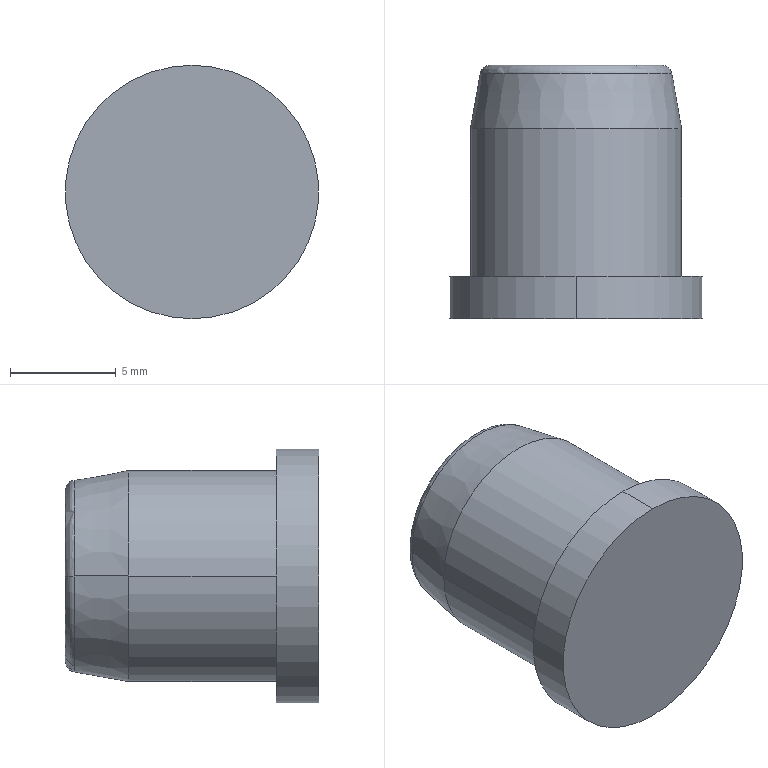Part | STEP file | 1519D3-2.stp.STEP | 1 solid | 12 faces | box 12 x 12 x 12 mm | volume 986.571 mm3 | cylinder 4 | plane 3 | cone 3 | torus 2 | commonest cylinder face diameters 10 x2 12 x2
STEP:
#1=CARTESIAN_POINT('',(0.,0.,6.));
#2=VERTEX_POINT('',#1);
#3=CARTESIAN_POINT('',(0.,0.,-6.));
#4=VERTEX_POINT('',#3);
#5=CARTESIAN_POINT('',(0.,0.,0.));
#6=DIRECTION('',(0.,-1.,0.));
#7=DIRECTION('',(0.,0.,1.));
#8=AXIS2_PLACEMENT_3D('',#5,#6,#7);
#9=CIRCLE('',#8,6.);
#10=EDGE_CURVE('',#2,#4,#9,.T.);
#11=ORIENTED_EDGE('',*,*,#10,.T.);
#12=CARTESIAN_POINT('',(0.,0.,0.));
#13=DIRECTION('',(0.,-1.,0.));
#14=DIRECTION('',(0.,0.,-1.));
#15=AXIS2_PLACEMENT_3D('',#12,#13,#14);
#16=CIRCLE('',#15,6.);
#17=EDGE_CURVE('',#4,#2,#16,.T.);
#18=ORIENTED_EDGE('',*,*,#17,.T.);
#19=EDGE_LOOP('',(#11,#18));
#20=FACE_OUTER_BOUND('',#19,.T.);
#21=CARTESIAN_POINT('',(0.,0.,0.));
#22=DIRECTION('',(0.,1.,0.));
#23=DIRECTION('',(1.,0.,0.));
#24=AXIS2_PLACEMENT_3D('',#21,#22,#23);
#25=PLANE('',#24);
#26=ADVANCED_FACE('',(#20),#25,.F.);
#27=CARTESIAN_POINT('',(0.,2.,-6.));
#28=VERTEX_POINT('',#27);
#29=CARTESIAN_POINT('',(0.,0.,-6.));
#30=DIRECTION('',(0.,1.,0.));
#31=VECTOR('',#30,1000.);
#32=LINE('',#29,#31);
#33=EDGE_CURVE('',#4,#28,#32,.T.);
#34=ORIENTED_EDGE('',*,*,#33,.T.);
#35=CARTESIAN_POINT('',(0.,2.,6.));
#36=VERTEX_POINT('',#35);
#37=CARTESIAN_POINT('',(0.,2.,0.));
#38=DIRECTION('',(0.,-1.,0.));
#39=DIRECTION('',(0.,0.,-1.));
#40=AXIS2_PLACEMENT_3D('',#37,#38,#39);
#41=CIRCLE('',#40,6.);
#42=EDGE_CURVE('',#28,#36,#41,.T.);
#43=ORIENTED_EDGE('',*,*,#42,.T.);
#44=CARTESIAN_POINT('',(0.,0.,6.));
#45=DIRECTION('',(0.,1.,0.));
#46=VECTOR('',#45,1000.);
#47=LINE('',#44,#46);
#48=EDGE_CURVE('',#2,#36,#47,.T.);
#49=ORIENTED_EDGE('',*,*,#48,.F.);
#50=ORIENTED_EDGE('',*,*,#17,.F.);
#51=EDGE_LOOP('',(#34,#43,#49,#50));
#52=FACE_OUTER_BOUND('',#51,.T.);
#53=CARTESIAN_POINT('',(0.,0.,0.));
#54=DIRECTION('',(0.,-1.,0.));
#55=DIRECTION('',(0.,0.,-1.));
#56=AXIS2_PLACEMENT_3D('',#53,#54,#55);
#57=CYLINDRICAL_SURFACE('',#56,6.);
#58=ADVANCED_FACE('',(#52),#57,.T.);
#59=ORIENTED_EDGE('',*,*,#48,.T.);
#60=CARTESIAN_POINT('',(0.,2.,0.));
#61=DIRECTION('',(0.,-1.,0.));
#62=DIRECTION('',(0.,0.,1.));
#63=AXIS2_PLACEMENT_3D('',#60,#61,#62);
#64=CIRCLE('',#63,6.);
#65=EDGE_CURVE('',#36,#28,#64,.T.);
#66=ORIENTED_EDGE('',*,*,#65,.T.);
#67=ORIENTED_EDGE('',*,*,#33,.F.);
#68=ORIENTED_EDGE('',*,*,#10,.F.);
#69=EDGE_LOOP('',(#59,#66,#67,#68));
#70=FACE_OUTER_BOUND('',#69,.T.);
#71=CARTESIAN_POINT('',(0.,0.,0.));
#72=DIRECTION('',(0.,-1.,0.));
#73=DIRECTION('',(0.,0.,-1.));
#74=AXIS2_PLACEMENT_3D('',#71,#72,#73);
#75=CYLINDRICAL_SURFACE('',#74,6.);
#76=ADVANCED_FACE('',(#70),#75,.T.);
#77=CARTESIAN_POINT('',(-5.,2.,0.));
#78=VERTEX_POINT('',#77);
#79=CARTESIAN_POINT('',(5.,2.,0.));
#80=VERTEX_POINT('',#79);
#81=CARTESIAN_POINT('',(0.,2.,0.));
#82=DIRECTION('',(0.,1.,0.));
#83=DIRECTION('',(-1.,0.,0.));
#84=AXIS2_PLACEMENT_3D('',#81,#82,#83);
#85=CIRCLE('',#84,5.);
#86=EDGE_CURVE('',#78,#80,#85,.T.);
#87=ORIENTED_EDGE('',*,*,#86,.F.);
#88=CARTESIAN_POINT('',(0.,2.,0.));
#89=DIRECTION('',(0.,1.,0.));
#90=DIRECTION('',(1.,0.,0.));
#91=AXIS2_PLACEMENT_3D('',#88,#89,#90);
#92=CIRCLE('',#91,5.);
#93=EDGE_CURVE('',#80,#78,#92,.T.);
#94=ORIENTED_EDGE('',*,*,#93,.F.);
#95=EDGE_LOOP('',(#87,#94));
#96=FACE_BOUND('',#95,.T.);
#97=ORIENTED_EDGE('',*,*,#65,.F.);
#98=ORIENTED_EDGE('',*,*,#42,.F.);
#99=EDGE_LOOP('',(#97,#98));
#100=FACE_OUTER_BOUND('',#99,.T.);
#101=CARTESIAN_POINT('',(0.,2.,0.));
#102=DIRECTION('',(0.,-1.,0.));
#103=DIRECTION('',(0.,0.,-1.));
#104=AXIS2_PLACEMENT_3D('',#101,#102,#103);
#105=PLANE('',#104);
#106=ADVANCED_FACE('',(#96,#100),#105,.F.);
#107=CARTESIAN_POINT('',(-5.,9.,0.));
#108=VERTEX_POINT('',#107);
#109=CARTESIAN_POINT('',(-5.,2.,0.));
#110=DIRECTION('',(0.,1.,0.));
#111=VECTOR('',#110,1000.);
#112=LINE('',#109,#111);
#113=EDGE_CURVE('',#78,#108,#112,.T.);
#114=ORIENTED_EDGE('',*,*,#113,.T.);
#115=CARTESIAN_POINT('',(0.,9.,-5.));
#116=VERTEX_POINT('',#115);
#117=CARTESIAN_POINT('',(0.,9.,0.));
#118=DIRECTION('',(0.,1.,0.));
#119=DIRECTION('',(1.,0.,0.));
#120=AXIS2_PLACEMENT_3D('',#117,#118,#119);
#121=CIRCLE('',#120,5.);
#122=EDGE_CURVE('',#116,#108,#121,.T.);
#123=ORIENTED_EDGE('',*,*,#122,.F.);
#124=CARTESIAN_POINT('',(5.,9.,0.));
#125=VERTEX_POINT('',#124);
#126=CARTESIAN_POINT('',(0.,9.,0.));
#127=DIRECTION('',(0.,1.,0.));
#128=DIRECTION('',(1.,0.,0.));
#129=AXIS2_PLACEMENT_3D('',#126,#127,#128);
#130=CIRCLE('',#129,5.);
#131=EDGE_CURVE('',#125,#116,#130,.T.);
#132=ORIENTED_EDGE('',*,*,#131,.F.);
#133=CARTESIAN_POINT('',(5.,2.,0.));
#134=DIRECTION('',(0.,1.,0.));
#135=VECTOR('',#134,1000.);
#136=LINE('',#133,#135);
#137=EDGE_CURVE('',#80,#125,#136,.T.);
#138=ORIENTED_EDGE('',*,*,#137,.F.);
#139=ORIENTED_EDGE('',*,*,#93,.T.);
#140=EDGE_LOOP('',(#114,#123,#132,#138,#139));
#141=FACE_OUTER_BOUND('',#140,.T.);
#142=CARTESIAN_POINT('',(0.,0.,0.));
#143=DIRECTION('',(0.,1.,0.));
#144=DIRECTION('',(1.,0.,0.));
#145=AXIS2_PLACEMENT_3D('',#142,#143,#144);
#146=CYLINDRICAL_SURFACE('',#145,5.);
#147=ADVANCED_FACE('',(#141),#146,.T.);
#148=ORIENTED_EDGE('',*,*,#137,.T.);
#149=CARTESIAN_POINT('',(0.,9.,0.));
#150=DIRECTION('',(0.,1.,0.));
#151=DIRECTION('',(-1.,0.,0.));
#152=AXIS2_PLACEMENT_3D('',#149,#150,#151);
#153=CIRCLE('',#152,5.);
#154=EDGE_CURVE('',#108,#125,#153,.T.);
#155=ORIENTED_EDGE('',*,*,#154,.F.);
#156=ORIENTED_EDGE('',*,*,#113,.F.);
#157=ORIENTED_EDGE('',*,*,#86,.T.);
#158=EDGE_LOOP('',(#148,#155,#156,#157));
#159=FACE_OUTER_BOUND('',#158,.T.);
#160=CARTESIAN_POINT('',(0.,0.,0.));
#161=DIRECTION('',(0.,1.,0.));
#162=DIRECTION('',(1.,0.,0.));
#163=AXIS2_PLACEMENT_3D('',#160,#161,#162);
#164=CYLINDRICAL_SURFACE('',#163,5.);
#165=ADVANCED_FACE('',(#159),#164,.T.);
#166=CARTESIAN_POINT('',(-4.544,11.587,0.000000001));
#167=VERTEX_POINT('',#166);
#168=CARTESIAN_POINT('',(-4.544,11.587,-0.000000004));
#169=DIRECTION('',(-0.1736,-0.9848,0.000000002));
#170=VECTOR('',#169,1000.);
#171=LINE('',#168,#170);
#172=EDGE_CURVE('',#167,#108,#171,.T.);
#173=ORIENTED_EDGE('',*,*,#172,.T.);
#174=ORIENTED_EDGE('',*,*,#154,.T.);
#175=CARTESIAN_POINT('',(4.544,11.587,-0.000000001));
#176=VERTEX_POINT('',#175);
#177=CARTESIAN_POINT('',(4.544,11.587,0.000000004));
#178=DIRECTION('',(0.1736,-0.9848,-0.000000002));
#179=VECTOR('',#178,1000.);
#180=LINE('',#177,#179);
#181=EDGE_CURVE('',#176,#125,#180,.T.);
#182=ORIENTED_EDGE('',*,*,#181,.F.);
#183=CARTESIAN_POINT('',(0.,11.587,0.));
#184=DIRECTION('',(0.,1.,0.));
#185=DIRECTION('',(-1.,0.,0.));
#186=AXIS2_PLACEMENT_3D('',#183,#184,#185);
#187=CIRCLE('',#186,4.544);
#188=EDGE_CURVE('',#167,#176,#187,.T.);
#189=ORIENTED_EDGE('',*,*,#188,.F.);
#190=EDGE_LOOP('',(#173,#174,#182,#189));
#191=FACE_OUTER_BOUND('',#190,.T.);
#192=CARTESIAN_POINT('',(0.,10.293,0.));
#193=DIRECTION('',(0.,-1.,0.));
#194=DIRECTION('',(0.,0.,-1.));
#195=AXIS2_PLACEMENT_3D('',#192,#193,#194);
#196=CONICAL_SURFACE('',#195,4.772,0.1745);
#197=ADVANCED_FACE('',(#191),#196,.T.);
#198=CARTESIAN_POINT('',(-4.051,12.,-0.000000008));
#199=VERTEX_POINT('',#198);
#200=CARTESIAN_POINT('',(-4.051,11.5,-0.000000008));
#201=DIRECTION('',(-0.000000002,0.,1.));
#202=DIRECTION('',(0.,1.,0.));
#203=AXIS2_PLACEMENT_3D('',#200,#201,#202);
#204=CIRCLE('',#203,0.5);
#205=EDGE_CURVE('',#199,#167,#204,.T.);
#206=ORIENTED_EDGE('',*,*,#205,.T.);
#207=ORIENTED_EDGE('',*,*,#188,.T.);
#208=CARTESIAN_POINT('',(4.051,12.,0.000000008));
#209=VERTEX_POINT('',#208);
#210=CARTESIAN_POINT('',(4.051,11.5,0.000000008));
#211=DIRECTION('',(0.000000002,0.,-1.));
#212=DIRECTION('',(0.,1.,0.));
#213=AXIS2_PLACEMENT_3D('',#210,#211,#212);
#214=CIRCLE('',#213,0.5);
#215=EDGE_CURVE('',#209,#176,#214,.T.);
#216=ORIENTED_EDGE('',*,*,#215,.F.);
#217=CARTESIAN_POINT('',(0.,12.,0.));
#218=DIRECTION('',(0.,1.,0.));
#219=DIRECTION('',(-1.,0.,-0.000000002));
#220=AXIS2_PLACEMENT_3D('',#217,#218,#219);
#221=CIRCLE('',#220,4.051);
#222=EDGE_CURVE('',#199,#209,#221,.T.);
#223=ORIENTED_EDGE('',*,*,#222,.F.);
#224=EDGE_LOOP('',(#206,#207,#216,#223));
#225=FACE_OUTER_BOUND('',#224,.T.);
#226=CARTESIAN_POINT('',(0.,11.5,0.));
#227=DIRECTION('',(0.,-1.,0.));
#228=DIRECTION('',(-1.,0.,-0.008557));
#229=AXIS2_PLACEMENT_3D('',#226,#227,#228);
#230=TOROIDAL_SURFACE('',#229,4.051,0.5);
#231=ADVANCED_FACE('',(#225),#230,.T.);
#232=CARTESIAN_POINT('',(0.,12.,0.));
#233=DIRECTION('',(0.,1.,0.));
#234=DIRECTION('',(1.,0.,0.000000002));
#235=AXIS2_PLACEMENT_3D('',#232,#233,#234);
#236=CIRCLE('',#235,4.051);
#237=EDGE_CURVE('',#209,#199,#236,.T.);
#238=ORIENTED_EDGE('',*,*,#237,.T.);
#239=ORIENTED_EDGE('',*,*,#222,.T.);
#240=EDGE_LOOP('',(#238,#239));
#241=FACE_OUTER_BOUND('',#240,.T.);
#242=CARTESIAN_POINT('',(0.,12.,0.));
#243=DIRECTION('',(0.,1.,0.));
#244=DIRECTION('',(1.,0.,0.));
#245=AXIS2_PLACEMENT_3D('',#242,#243,#244);
#246=PLANE('',#245);
#247=ADVANCED_FACE('',(#241),#246,.T.);
#248=ORIENTED_EDGE('',*,*,#215,.T.);
#249=CARTESIAN_POINT('',(0.,11.587,-4.544));
#250=VERTEX_POINT('',#249);
#251=CARTESIAN_POINT('',(0.,11.587,0.));
#252=DIRECTION('',(0.,1.,0.));
#253=DIRECTION('',(1.,0.,0.));
#254=AXIS2_PLACEMENT_3D('',#251,#252,#253);
#255=CIRCLE('',#254,4.544);
#256=EDGE_CURVE('',#176,#250,#255,.T.);
#257=ORIENTED_EDGE('',*,*,#256,.T.);
#258=CARTESIAN_POINT('',(0.,11.587,0.));
#259=DIRECTION('',(0.,1.,0.));
#260=DIRECTION('',(1.,0.,0.));
#261=AXIS2_PLACEMENT_3D('',#258,#259,#260);
#262=CIRCLE('',#261,4.544);
#263=EDGE_CURVE('',#250,#167,#262,.T.);
#264=ORIENTED_EDGE('',*,*,#263,.T.);
#265=ORIENTED_EDGE('',*,*,#205,.F.);
#266=ORIENTED_EDGE('',*,*,#237,.F.);
#267=EDGE_LOOP('',(#248,#257,#264,#265,#266));
#268=FACE_OUTER_BOUND('',#267,.T.);
#269=CARTESIAN_POINT('',(0.,11.5,0.));
#270=DIRECTION('',(0.,-1.,0.));
#271=DIRECTION('',(1.,0.,0.008557));
#272=AXIS2_PLACEMENT_3D('',#269,#270,#271);
#273=TOROIDAL_SURFACE('',#272,4.051,0.5);
#274=ADVANCED_FACE('',(#268),#273,.T.);
#275=CARTESIAN_POINT('',(0.,10.293,-4.772));
#276=DIRECTION('',(0.,-0.9848,-0.1736));
#277=VECTOR('',#276,1000.);
#278=LINE('',#275,#277);
#279=EDGE_CURVE('',#250,#116,#278,.T.);
#280=ORIENTED_EDGE('',*,*,#279,.F.);
#281=ORIENTED_EDGE('',*,*,#256,.F.);
#282=ORIENTED_EDGE('',*,*,#181,.T.);
#283=ORIENTED_EDGE('',*,*,#131,.T.);
#284=EDGE_LOOP('',(#280,#281,#282,#283));
#285=FACE_OUTER_BOUND('',#284,.T.);
#286=CARTESIAN_POINT('',(0.,10.293,0.));
#287=DIRECTION('',(0.,-1.,0.));
#288=DIRECTION('',(0.,0.,-1.));
#289=AXIS2_PLACEMENT_3D('',#286,#287,#288);
#290=CONICAL_SURFACE('',#289,4.772,0.1745);
#291=ADVANCED_FACE('',(#285),#290,.T.);
#292=ORIENTED_EDGE('',*,*,#263,.F.);
#293=ORIENTED_EDGE('',*,*,#279,.T.);
#294=ORIENTED_EDGE('',*,*,#122,.T.);
#295=ORIENTED_EDGE('',*,*,#172,.F.);
#296=EDGE_LOOP('',(#292,#293,#294,#295));
#297=FACE_OUTER_BOUND('',#296,.T.);
#298=CARTESIAN_POINT('',(0.,10.293,0.));
#299=DIRECTION('',(0.,-1.,0.));
#300=DIRECTION('',(0.,0.,-1.));
#301=AXIS2_PLACEMENT_3D('',#298,#299,#300);
#302=CONICAL_SURFACE('',#301,4.772,0.1745);
#303=ADVANCED_FACE('',(#297),#302,.T.);
#304=CLOSED_SHELL('',(#26,#58,#76,#106,#147,#165,#197,#231,#247,#274,#291,#303));
#305=MANIFOLD_SOLID_BREP('',#304);
#306=CARTESIAN_POINT('',(0.,0.,0.));
#307=DIRECTION('',(0.,0.,1.));
#308=DIRECTION('',(1.,0.,0.));
#309=AXIS2_PLACEMENT_3D('',#306,#307,#308);
#310=(LENGTH_UNIT()NAMED_UNIT(*)SI_UNIT(.MILLI.,.METRE.));
#311=UNCERTAINTY_MEASURE_WITH_UNIT(LENGTH_MEASURE(0.00001),#310,'','');
#312=(NAMED_UNIT(*)PLANE_ANGLE_UNIT()SI_UNIT($,.RADIAN.));
#313=(NAMED_UNIT(*)SI_UNIT($,.STERADIAN.)SOLID_ANGLE_UNIT());
#314=(GEOMETRIC_REPRESENTATION_CONTEXT(3)GLOBAL_UNCERTAINTY_ASSIGNED_CONTEXT((#311))GLOBAL_UNIT_ASSIGNED_CONTEXT((#310,#312,#313))REPRESENTATION_CONTEXT('',''));
#315=ADVANCED_BREP_SHAPE_REPRESENTATION('',(#305,#309),#314);